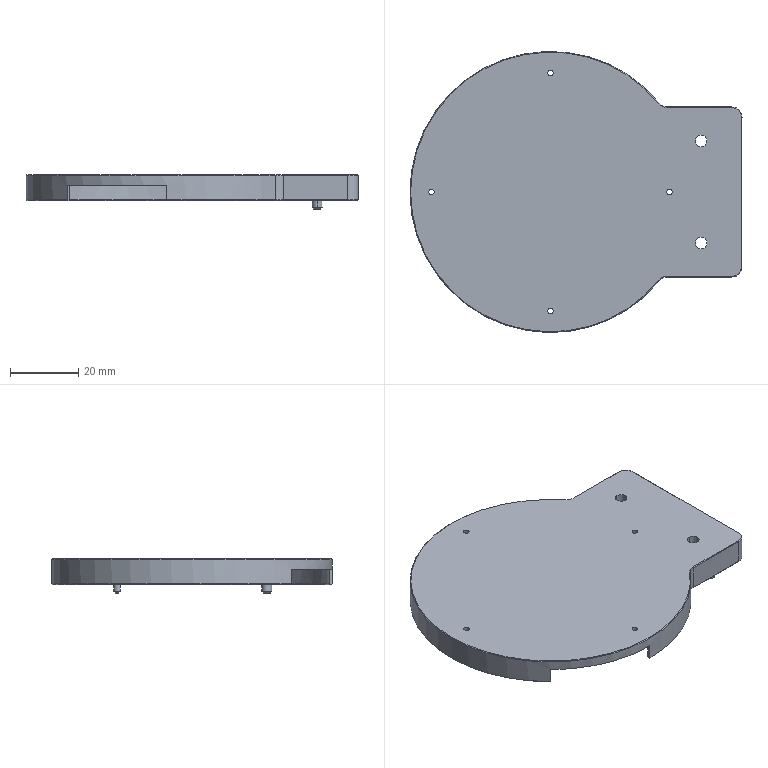NC program | NX | posted with a generic post | part box 97.6 x 82.6 x 10 mm
Whole program:
N10 G17 G21 G94 G90
(DRILLING_COPY_1 , TOOL : D6A45)
N12 T01 M6
N14 G54
N16 G17 G0 G90 X-42.5 Y0. S5000 M3
N18 G43 Z30. H1
N20 G94 G81 G98 Z-1.1 F350. R3.
N22 X-7.5 Y-35.
N24 X36.8 Y-15.
N26 X27.5 Y0.
N28 X36.8 Y15.
N30 X-7.5 Y35.
N32 G80
N34 G0 X-7.5 Y35. Z30.
N36 M5
(DRILLING_COPY_1_COPY_COPY , TOOL : 1.6ZT)
N38 T16 M6
N40 G54
N42 G17 G0 G90 X27.5 Y0. S2000 M3
N44 G43 Z30. H16
N46 G94 G83 G98 Z-4.981 F150. Q2. R3.
N48 X-7.5 Y35.
N50 X-42.5 Y0.
N52 X-7.5 Y-35.
N54 G80
N56 G0 X-7.5 Y-35. Z30.
N58 M5
(DRILLING_COPY_1_COPY_1_1_COPY_1 , TOOL : 3.4ZT)
N60 T03 M6
N62 G54
N64 G17 G0 G90 X36.8 Y15. S2000 M3
N66 G43 Z30. H3
N68 G94 G83 G98 Z-10.021 F200. Q2. R3.
N70 Y-15.
N72 G80
N74 G0 X36.8 Y-15. Z30.
N76 M5
(ZLEVEL_PROFILE , TOOL : D10)
N78 T15 M6
N80 G54
N82 G17 G0 G90 X33.985 Y30.1 S9500 M3
N84 G43 Z30. H15
N86 Z1.5
N88 G94 G1 X45.8 Z0.881 F1000.
N90 X46.498 Z0.844
N92 X48.35 Y29.72 Z0.745
N94 X50.065 Y28.921 Z0.646
N96 X51.549 Y27.749 Z0.547
N98 X52.721 Y26.265 Z0.448
N100 X53.52 Y24.55 Z0.349
N102 X53.9 Y22.698 Z0.25
N104 Y22. Z0.213
N106 Y0. Z-0.94
N108 Y-22. F3200.
N110 G2 X45.8 Y-30.1 R8.1
N112 G1 X27.812
N114 G2 X27.812 Y30.1 R-46.4
N116 G1 X45.8
N118 G2 X53.9 Y22. R8.1
N120 G1 Y0.
N122 Y-21.541 Z-1.316
N124 Y-21.926 Z-1.323
N126 X53.894 Y-22.31 Z-1.329
N128 X53.87 Y-22.694 Z-1.336
N130 X53.828 Y-23.076 Z-1.343
N132 X53.768 Y-23.456 Z-1.35
N134 X53.69 Y-23.833 Z-1.356
N136 X53.594 Y-24.205 Z-1.363
N138 X53.48 Y-24.573 Z-1.37
N140 X53.35 Y-24.935 Z-1.376
N142 X53.202 Y-25.29 Z-1.383
N144 X53.037 Y-25.637 Z-1.39
N146 X52.857 Y-25.977 Z-1.397
N148 X52.66 Y-26.307 Z-1.403
N150 X52.448 Y-26.628 Z-1.41
N152 X52.22 Y-26.939 Z-1.417
N154 X51.979 Y-27.238 Z-1.423
N156 X51.723 Y-27.525 Z-1.43
N158 X51.454 Y-27.8 Z-1.437
N160 X51.172 Y-28.062 Z-1.444
N162 X50.879 Y-28.31 Z-1.45
N164 X50.573 Y-28.544 Z-1.457
N166 X50.257 Y-28.763 Z-1.464
N168 X49.931 Y-28.967 Z-1.47
N170 X49.596 Y-29.156 Z-1.477
N172 X49.252 Y-29.328 Z-1.484
N174 X48.9 Y-29.483 Z-1.491
N176 X48.541 Y-29.622 Z-1.497
N178 X48.176 Y-29.744 Z-1.504
N180 X47.806 Y-29.848 Z-1.511
N182 X47.431 Y-29.934 Z-1.517
N184 X47.053 Y-30.003 Z-1.524
N186 X46.672 Y-30.053 Z-1.531
N188 X46.288 Y-30.085 Z-1.538
N190 X45.904 Y-30.099 Z-1.544
N192 X45.519 Y-30.1 Z-1.551
N194 X28.21 Z-1.853
N196 X27.818 Z-1.86
N198 X27.57 Y-30.382 Z-1.867
N200 X27.317 Y-30.672 Z-1.873
N202 X27.061 Y-30.959 Z-1.88
N204 G2 X27.812 Y30.1 R-46.4
N206 G1 X45.8
N208 G2 X53.9 Y22. R8.1
N210 G1 Y0.
N212 Y-21.541 Z-2.256
N214 Y-21.926 Z-2.263
N216 X53.894 Y-22.31 Z-2.269
N218 X53.87 Y-22.694 Z-2.276
N220 X53.828 Y-23.076 Z-2.283
N222 X53.768 Y-23.456 Z-2.29
N224 X53.69 Y-23.833 Z-2.296
N226 X53.594 Y-24.205 Z-2.303
N228 X53.48 Y-24.573 Z-2.31
N230 X53.35 Y-24.935 Z-2.316
N232 X53.202 Y-25.29 Z-2.323
N234 X53.037 Y-25.637 Z-2.33
N236 X52.857 Y-25.977 Z-2.337
N238 X52.66 Y-26.307 Z-2.343
N240 X52.448 Y-26.628 Z-2.35
N242 X52.22 Y-26.939 Z-2.357
N244 X51.979 Y-27.238 Z-2.363
N246 X51.723 Y-27.525 Z-2.37
N248 X51.454 Y-27.8 Z-2.377
N250 X51.172 Y-28.062 Z-2.384
N252 X50.879 Y-28.31 Z-2.39
N254 X50.573 Y-28.544 Z-2.397
N256 X50.257 Y-28.763 Z-2.404
N258 X49.931 Y-28.967 Z-2.41
N260 X49.596 Y-29.156 Z-2.417
N262 X49.252 Y-29.328 Z-2.424
N264 X48.9 Y-29.483 Z-2.431
N266 X48.541 Y-29.622 Z-2.437
N268 X48.176 Y-29.744 Z-2.444
N270 X47.806 Y-29.848 Z-2.451
N272 X47.431 Y-29.934 Z-2.457
N274 X47.053 Y-30.003 Z-2.464
N276 X46.672 Y-30.053 Z-2.471
N278 X46.288 Y-30.085 Z-2.478
N280 X45.904 Y-30.099 Z-2.484
N282 X45.519 Y-30.1 Z-2.491
N284 X28.21 Z-2.793
N286 X27.818 Z-2.8
N288 X27.57 Y-30.382 Z-2.807
N290 X27.317 Y-30.672 Z-2.813
N292 X27.061 Y-30.959 Z-2.82
N294 G2 X27.812 Y30.1 R-46.4
N296 G1 X45.8
N298 G2 X53.9 Y22. R8.1
N300 G1 Y0.
N302 Y-21.541 Z-3.196
N304 Y-21.926 Z-3.203
N306 X53.894 Y-22.31 Z-3.209
N308 X53.87 Y-22.694 Z-3.216
N310 X53.828 Y-23.076 Z-3.223
N312 X53.768 Y-23.456 Z-3.23
N314 X53.69 Y-23.833 Z-3.236
N316 X53.594 Y-24.205 Z-3.243
N318 X53.48 Y-24.573 Z-3.25
N320 X53.35 Y-24.935 Z-3.256
N322 X53.202 Y-25.29 Z-3.263
N324 X53.037 Y-25.637 Z-3.27
N326 X52.857 Y-25.977 Z-3.277
N328 X52.66 Y-26.307 Z-3.283
N330 X52.448 Y-26.628 Z-3.29
N332 X52.22 Y-26.939 Z-3.297
N334 X51.979 Y-27.238 Z-3.303
N336 X51.723 Y-27.525 Z-3.31
N338 X51.454 Y-27.8 Z-3.317
N340 X51.172 Y-28.062 Z-3.324
N342 X50.879 Y-28.31 Z-3.33
N344 X50.573 Y-28.544 Z-3.337
N346 X50.257 Y-28.763 Z-3.344
N348 X49.931 Y-28.967 Z-3.35
N350 X49.596 Y-29.156 Z-3.357
N352 X49.252 Y-29.328 Z-3.364
N354 X48.9 Y-29.483 Z-3.371
N356 X48.541 Y-29.622 Z-3.377
N358 X48.176 Y-29.744 Z-3.384
N360 X47.806 Y-29.848 Z-3.391
N362 X47.431 Y-29.934 Z-3.397
N364 X47.053 Y-30.003 Z-3.404
N366 X46.672 Y-30.053 Z-3.411
N368 X46.288 Y-30.085 Z-3.418
N370 X45.904 Y-30.099 Z-3.424
N372 X45.519 Y-30.1 Z-3.431
N374 X28.21 Z-3.733
N376 X27.818 Z-3.74
N378 X27.57 Y-30.382 Z-3.747
N380 X27.317 Y-30.672 Z-3.753
N382 X27.061 Y-30.959 Z-3.76
N384 G2 X27.812 Y30.1 R-46.4
N386 G1 X45.8
N388 G2 X53.9 Y22. R8.1
N390 G1 Y0.
N392 Y-21.541 Z-4.136
N394 Y-21.926 Z-4.143
N396 X53.894 Y-22.31 Z-4.149
N398 X53.87 Y-22.694 Z-4.156
N400 X53.828 Y-23.076 Z-4.163
N402 X53.768 Y-23.456 Z-4.17
N404 X53.69 Y-23.833 Z-4.176
N406 X53.594 Y-24.205 Z-4.183
N408 X53.48 Y-24.573 Z-4.19
N410 X53.35 Y-24.935 Z-4.196
N412 X53.202 Y-25.29 Z-4.203
N414 X53.037 Y-25.637 Z-4.21
N416 X52.857 Y-25.977 Z-4.217
N418 X52.66 Y-26.307 Z-4.223
N420 X52.448 Y-26.628 Z-4.23
N422 X52.22 Y-26.939 Z-4.237
N424 X51.979 Y-27.238 Z-4.243
N426 X51.723 Y-27.525 Z-4.25
N428 X51.454 Y-27.8 Z-4.257
N430 X51.172 Y-28.062 Z-4.264
N432 X50.879 Y-28.31 Z-4.27
N434 X50.573 Y-28.544 Z-4.277
N436 X50.257 Y-28.763 Z-4.284
N438 X49.931 Y-28.967 Z-4.29
N440 X49.596 Y-29.156 Z-4.297
N442 X49.252 Y-29.328 Z-4.304
N444 X48.9 Y-29.483 Z-4.311
N446 X48.541 Y-29.622 Z-4.317
N448 X48.176 Y-29.744 Z-4.324
N450 X47.806 Y-29.848 Z-4.331
N452 X47.431 Y-29.934 Z-4.337
N454 X47.053 Y-30.003 Z-4.344
N456 X46.672 Y-30.053 Z-4.351
N458 X46.288 Y-30.085 Z-4.358
N460 X45.904 Y-30.099 Z-4.364
N462 X45.519 Y-30.1 Z-4.371
N464 X28.21 Z-4.673
N466 X27.818 Z-4.68
N468 X27.57 Y-30.382 Z-4.687
N470 X27.317 Y-30.672 Z-4.693
N472 X27.061 Y-30.959 Z-4.7
N474 G2 X27.812 Y30.1 R-46.4
N476 G1 X45.8
N478 G2 X53.9 Y22. R8.1
N480 G1 Y0.
N482 Y-21.541 Z-5.076
N484 Y-21.926 Z-5.083
N486 X53.894 Y-22.31 Z-5.089
N488 X53.87 Y-22.694 Z-5.096
N490 X53.828 Y-23.076 Z-5.103
N492 X53.768 Y-23.456 Z-5.11
N494 X53.69 Y-23.833 Z-5.116
N496 X53.594 Y-24.205 Z-5.123
N498 X53.48 Y-24.573 Z-5.13
N500 X53.35 Y-24.935 Z-5.136
N502 X53.202 Y-25.29 Z-5.143
N504 X53.037 Y-25.637 Z-5.15
N506 X52.857 Y-25.977 Z-5.157
N508 X52.66 Y-26.307 Z-5.163
N510 X52.448 Y-26.628 Z-5.17
N512 X52.22 Y-26.939 Z-5.177
N514 X51.979 Y-27.238 Z-5.183
N516 X51.723 Y-27.525 Z-5.19
N518 X51.454 Y-27.8 Z-5.197
N520 X51.172 Y-28.062 Z-5.204
N522 X50.879 Y-28.31 Z-5.21
N524 X50.573 Y-28.544 Z-5.217
N526 X50.257 Y-28.763 Z-5.224
N528 X49.931 Y-28.967 Z-5.23
N530 X49.596 Y-29.156 Z-5.237
N532 X49.252 Y-29.328 Z-5.244
N534 X48.9 Y-29.483 Z-5.251
N536 X48.541 Y-29.622 Z-5.257
N538 X48.176 Y-29.744 Z-5.264
N540 X47.806 Y-29.848 Z-5.271
N542 X47.431 Y-29.934 Z-5.277
N544 X47.053 Y-30.003 Z-5.284
N546 X46.672 Y-30.053 Z-5.291
N548 X46.288 Y-30.085 Z-5.298
N550 X45.904 Y-30.099 Z-5.304
N552 X45.519 Y-30.1 Z-5.311
N554 X28.21 Z-5.613
N556 X27.818 Z-5.62
N558 X27.57 Y-30.382 Z-5.627
N560 X27.317 Y-30.672 Z-5.633
N562 X27.061 Y-30.959 Z-5.64
N564 G2 X27.812 Y30.1 R-46.4
N566 G1 X45.8
N568 G2 X53.9 Y22. R8.1
N570 G1 Y0.
N572 Y-21.541 Z-6.016
N574 Y-21.926 Z-6.023
N576 X53.894 Y-22.31 Z-6.029
N578 X53.87 Y-22.694 Z-6.036
N580 X53.828 Y-23.076 Z-6.043
N582 X53.768 Y-23.456 Z-6.05
N584 X53.69 Y-23.833 Z-6.056
N586 X53.594 Y-24.205 Z-6.063
N588 X53.48 Y-24.573 Z-6.07
N590 X53.35 Y-24.935 Z-6.076
N592 X53.202 Y-25.29 Z-6.083
N594 X53.037 Y-25.637 Z-6.09
N596 X52.857 Y-25.977 Z-6.097
N598 X52.66 Y-26.307 Z-6.103
N600 X52.448 Y-26.628 Z-6.11
N602 X52.22 Y-26.939 Z-6.117
N604 X51.979 Y-27.238 Z-6.123
N606 X51.723 Y-27.525 Z-6.13
N608 X51.454 Y-27.8 Z-6.137
N610 X51.172 Y-28.062 Z-6.144
N612 X50.879 Y-28.31 Z-6.15
N614 X50.573 Y-28.544 Z-6.157
N616 X50.257 Y-28.763 Z-6.164
N618 X49.931 Y-28.967 Z-6.17
N620 X49.596 Y-29.156 Z-6.177
N622 X49.252 Y-29.328 Z-6.184
N624 X48.9 Y-29.483 Z-6.191
N626 X48.541 Y-29.622 Z-6.197
N628 X48.176 Y-29.744 Z-6.204
N630 X47.806 Y-29.848 Z-6.211
N632 X47.431 Y-29.934 Z-6.217
N634 X47.053 Y-30.003 Z-6.224
N636 X46.672 Y-30.053 Z-6.231
N638 X46.288 Y-30.085 Z-6.238
N640 X45.904 Y-30.099 Z-6.244
N642 X45.519 Y-30.1 Z-6.251
N644 X28.21 Z-6.553
N646 X27.818 Z-6.56
N648 X27.57 Y-30.382 Z-6.567
N650 X27.317 Y-30.672 Z-6.573
N652 X27.061 Y-30.959 Z-6.58
N654 G2 X27.812 Y30.1 R-46.4
N656 G1 X45.8
N658 G2 X53.9 Y22. R8.1
N660 G1 Y0.
N662 Y-21.541 Z-6.956
N664 Y-21.926 Z-6.963
N666 X53.894 Y-22.31 Z-6.969
N668 X53.87 Y-22.694 Z-6.976
N670 X53.828 Y-23.076 Z-6.983
N672 X53.768 Y-23.456 Z-6.99
N674 X53.69 Y-23.833 Z-6.996
N676 X53.594 Y-24.205 Z-7.003
N678 X53.48 Y-24.573 Z-7.01
N680 X53.35 Y-24.935 Z-7.016
N682 X53.202 Y-25.29 Z-7.023
N684 X53.037 Y-25.637 Z-7.03
N686 X52.857 Y-25.977 Z-7.037
N688 X52.66 Y-26.307 Z-7.043
N690 X52.448 Y-26.628 Z-7.05
N692 X52.22 Y-26.939 Z-7.057
N694 X51.979 Y-27.238 Z-7.063
N696 X51.723 Y-27.525 Z-7.07
N698 X51.454 Y-27.8 Z-7.077
N700 X51.172 Y-28.062 Z-7.084
N702 X50.879 Y-28.31 Z-7.09
N704 X50.573 Y-28.544 Z-7.097
N706 X50.257 Y-28.763 Z-7.104
N708 X49.931 Y-28.967 Z-7.11
N710 X49.596 Y-29.156 Z-7.117
N712 X49.252 Y-29.328 Z-7.124
N714 X48.9 Y-29.483 Z-7.131
N716 X48.541 Y-29.622 Z-7.137
N718 X48.176 Y-29.744 Z-7.144
N720 X47.806 Y-29.848 Z-7.151
N722 X47.431 Y-29.934 Z-7.157
N724 X47.053 Y-30.003 Z-7.164
N726 X46.672 Y-30.053 Z-7.171
N728 X46.288 Y-30.085 Z-7.178
N730 X45.904 Y-30.099 Z-7.184
N732 X45.519 Y-30.1 Z-7.191
N734 X28.21 Z-7.493
N736 X27.818 Z-7.5
N738 X27.57 Y-30.382 Z-7.507
N740 X27.317 Y-30.672 Z-7.513
N742 X27.061 Y-30.959 Z-7.52
N744 G2 X27.812 Y30.1 R-46.4
N746 G1 X45.8
N748 G2 X53.9 Y22. R8.1
N750 G1 Y0.
N752 Y-21.541 Z-7.896
N754 Y-21.926 Z-7.903
N756 X53.894 Y-22.31 Z-7.909
N758 X53.87 Y-22.694 Z-7.916
N760 X53.828 Y-23.076 Z-7.923
N762 X53.768 Y-23.456 Z-7.93
N764 X53.69 Y-23.833 Z-7.936
N766 X53.594 Y-24.205 Z-7.943
N768 X53.48 Y-24.573 Z-7.95
N770 X53.35 Y-24.935 Z-7.956
N772 X53.202 Y-25.29 Z-7.963
N774 X53.037 Y-25.637 Z-7.97
N776 X52.857 Y-25.977 Z-7.977
N778 X52.66 Y-26.307 Z-7.983
N780 X52.448 Y-26.628 Z-7.99
N782 X52.22 Y-26.939 Z-7.997
N784 X51.979 Y-27.238 Z-8.003
N786 X51.723 Y-27.525 Z-8.01
N788 X51.454 Y-27.8 Z-8.017
N790 X51.172 Y-28.062 Z-8.024
N792 X50.879 Y-28.31 Z-8.03
N794 X50.573 Y-28.544 Z-8.037
N796 X50.257 Y-28.763 Z-8.044
N798 X49.931 Y-28.967 Z-8.05
N800 X49.596 Y-29.156 Z-8.057
N802 X49.252 Y-29.328 Z-8.064
N804 X48.9 Y-29.483 Z-8.071
N806 X48.541 Y-29.622 Z-8.077
N808 X48.176 Y-29.744 Z-8.084
N810 X47.806 Y-29.848 Z-8.091
N812 X47.431 Y-29.934 Z-8.097
N814 X47.053 Y-30.003 Z-8.104
N816 X46.672 Y-30.053 Z-8.111
N818 X46.288 Y-30.085 Z-8.118
N820 X45.904 Y-30.099 Z-8.124
N822 X45.519 Y-30.1 Z-8.131
N824 X28.21 Z-8.433
N826 X27.818 Z-8.44
N828 X27.57 Y-30.382 Z-8.447
N830 X27.317 Y-30.672 Z-8.453
N832 X27.061 Y-30.959 Z-8.46
N834 G2 X27.812 Y30.1 R-46.4
N836 G1 X45.8
N838 G2 X53.9 Y22. R8.1
N840 G1 Y0.
N842 Y-21.541 Z-8.836
N844 Y-21.926 Z-8.843
N846 X53.894 Y-22.31 Z-8.849
N848 X53.87 Y-22.694 Z-8.856
N850 X53.828 Y-23.076 Z-8.863
N852 X53.768 Y-23.456 Z-8.87
N854 X53.69 Y-23.833 Z-8.876
N856 X53.594 Y-24.205 Z-8.883
N858 X53.48 Y-24.573 Z-8.89
N860 X53.35 Y-24.935 Z-8.896
N862 X53.202 Y-25.29 Z-8.903
N864 X53.037 Y-25.637 Z-8.91
N866 X52.857 Y-25.977 Z-8.917
N868 X52.66 Y-26.307 Z-8.923
N870 X52.448 Y-26.628 Z-8.93
N872 X52.22 Y-26.939 Z-8.937
N874 X51.979 Y-27.238 Z-8.943
N876 X51.723 Y-27.525 Z-8.95
N878 X51.454 Y-27.8 Z-8.957
N880 X51.172 Y-28.062 Z-8.964
N882 X50.879 Y-28.31 Z-8.97
N884 X50.573 Y-28.544 Z-8.977
N886 X50.257 Y-28.763 Z-8.984
N888 X49.931 Y-28.967 Z-8.99
N890 X49.596 Y-29.156 Z-8.997
N892 X49.252 Y-29.328 Z-9.004
N894 X48.9 Y-29.483 Z-9.011
N896 X48.541 Y-29.622 Z-9.017
N898 X48.176 Y-29.744 Z-9.024
N900 X47.806 Y-29.848 Z-9.031
N902 X47.431 Y-29.934 Z-9.037
N904 X47.053 Y-30.003 Z-9.044
N906 X46.672 Y-30.053 Z-9.051
N908 X46.288 Y-30.085 Z-9.058
N910 X45.904 Y-30.099 Z-9.064
N912 X45.519 Y-30.1 Z-9.071
N914 X28.21 Z-9.373
N916 X27.818 Z-9.38
N918 X27.57 Y-30.382 Z-9.387
N920 X27.317 Y-30.672 Z-9.393
N922 X27.061 Y-30.959 Z-9.4
N924 G2 X27.812 Y30.1 R-46.4
N926 G1 X45.8
N928 G2 X53.9 Y22. R8.1
N930 G1 Y-22.
N932 G2 X45.8 Y-30.1 R8.1
N934 G1 X27.812
N936 G2 X27.061 Y-30.959 R46.4
N938 G1 Z-7.9
N940 G0 Z30.
N942 M5
(ZLEVEL_PROFILE_2 , TOOL : D6)
N944 T12 M6
N946 G54
N948 G17 G0 G90 X26.467 Y30.274 S9500 M3
N950 G43 Z30. H12
N952 Z-0.5
N954 G94 G1 X26.123 Y29.307 F1600.
N956 G3 X26.231 Y28.717 R0.6
N958 G2 X26.829 Y28. R44.3
N960 G1 X27.772
N962 G3 X28.292 Y28.3 R0.6
N964 G1 X28.812 Y29.2
N966 G0 X26.467 Y30.274 Z-1.
N968 G1 X26.123 Y29.307
N970 G3 X26.231 Y28.717 R0.6
N972 G2 X26.829 Y28. R44.3
N974 G1 X27.772
N976 G3 X28.292 Y28.3 R0.6
N978 G1 X28.812 Y29.2
N980 G0 X26.467 Y30.274 Z-1.5
N982 G1 X26.123 Y29.307
N984 G3 X26.231 Y28.717 R0.6
N986 G2 X26.829 Y28. R44.3
N988 G1 X27.772
N990 G3 X28.292 Y28.3 R0.6
N992 G1 X28.812 Y29.2
N994 G0 X26.467 Y30.274 Z-2.
N996 G1 X26.123 Y29.307
N998 G3 X26.231 Y28.717 R0.6
N1000 G2 X26.829 Y28. R44.3
N1002 G1 X27.772
N1004 G3 X28.292 Y28.3 R0.6
N1006 G1 X28.812 Y29.2
N1008 G0 X26.467 Y30.274 Z-2.5
N1010 G1 X26.123 Y29.307
N1012 G3 X26.231 Y28.717 R0.6
N1014 G2 X26.829 Y28. R44.3
N1016 G1 X27.772
N1018 G3 X28.292 Y28.3 R0.6
N1020 G1 X28.812 Y29.2
N1022 G0 X26.467 Y30.274 Z-3.
N1024 G1 X26.123 Y29.307
N1026 G3 X26.231 Y28.717 R0.6
N1028 G2 X26.829 Y28. R44.3
N1030 G1 X27.772
N1032 G3 X28.292 Y28.3 R0.6
N1034 G1 X28.812 Y29.2
N1036 G0 X26.467 Y30.274 Z-3.5
N1038 G1 X26.123 Y29.307
N1040 G3 X26.231 Y28.717 R0.6
N1042 G2 X26.829 Y28. R44.3
N1044 G1 X27.772
N1046 G3 X28.292 Y28.3 R0.6
N1048 G1 X28.812 Y29.2
N1050 G0 X26.467 Y30.274 Z-4.
N1052 G1 X26.123 Y29.307
N1054 G3 X26.231 Y28.717 R0.6
N1056 G2 X26.829 Y28. R44.3
N1058 G1 X27.772
N1060 G3 X28.292 Y28.3 R0.6
N1062 G1 X28.812 Y29.2
N1064 G0 X26.467 Y30.274 Z-4.5
N1066 G1 X26.123 Y29.307
N1068 G3 X26.231 Y28.717 R0.6
N1070 G2 X26.829 Y28. R44.3
N1072 G1 X27.772
N1074 G3 X28.292 Y28.3 R0.6
N1076 G1 X28.812 Y29.2
N1078 G0 X26.467 Y30.274 Z-5.
N1080 G1 X26.123 Y29.307
N1082 G3 X26.231 Y28.717 R0.6
N1084 G2 X26.829 Y28. R44.3
N1086 G1 X27.772
N1088 G3 X28.292 Y28.3 R0.6
N1090 G1 X28.812 Y29.2
N1092 G0 X26.467 Y30.274 Z-5.5
N1094 G1 X26.123 Y29.307
N1096 G3 X26.231 Y28.717 R0.6
N1098 G2 X26.829 Y28. R44.3
N1100 G1 X27.772
N1102 G3 X28.292 Y28.3 R0.6
N1104 G1 X28.812 Y29.2
N1106 G0 X26.467 Y30.274 Z-6.
N1108 G1 X26.123 Y29.307
N1110 G3 X26.231 Y28.717 R0.6
N1112 G2 X26.829 Y28. R44.3
N1114 G1 X27.772
N1116 G3 X28.292 Y28.3 R0.6
N1118 G1 X28.812 Y29.2
N1120 G0 X26.467 Y30.274 Z-6.5
N1122 G1 X26.123 Y29.307
N1124 G3 X26.231 Y28.717 R0.6
N1126 G2 X26.829 Y28. R44.3
N1128 G1 X27.772
N1130 G3 X28.292 Y28.3 R0.6
N1132 G1 X28.812 Y29.2
N1134 G0 X26.467 Y30.274 Z-7.
N1136 G1 X26.123 Y29.307
N1138 G3 X26.231 Y28.717 R0.6
N1140 G2 X26.829 Y28. R44.3
N1142 G1 X27.772
N1144 G3 X28.292 Y28.3 R0.6
N1146 G1 X28.812 Y29.2
N1148 G0 Z30.
N1150 Y-29.2
N1152 Z-0.5
N1154 G1 X28.292 Y-28.3
N1156 G3 X27.772 Y-28. R0.6
N1158 G1 X26.829
N1160 G2 X26.231 Y-28.717 R44.3
N1162 G3 X26.123 Y-29.307 R0.6
N1164 G1 X26.467 Y-30.274
N1166 G0 X28.812 Y-29.2 Z-1.
N1168 G1 X28.292 Y-28.3
N1170 G3 X27.772 Y-28. R0.6
N1172 G1 X26.829
N1174 G2 X26.231 Y-28.717 R44.3
N1176 G3 X26.123 Y-29.307 R0.6
N1178 G1 X26.467 Y-30.274
N1180 G0 X28.812 Y-29.2 Z-1.5
N1182 G1 X28.292 Y-28.3
N1184 G3 X27.772 Y-28. R0.6
N1186 G1 X26.829
N1188 G2 X26.231 Y-28.717 R44.3
N1190 G3 X26.123 Y-29.307 R0.6
N1192 G1 X26.467 Y-30.274
N1194 G0 X28.812 Y-29.2 Z-2.
N1196 G1 X28.292 Y-28.3
N1198 G3 X27.772 Y-28. R0.6
N1200 G1 X26.829
N1202 G2 X26.231 Y-28.717 R44.3
N1204 G3 X26.123 Y-29.307 R0.6
N1206 G1 X26.467 Y-30.274
N1208 G0 X28.812 Y-29.2 Z-2.5
N1210 G1 X28.292 Y-28.3
N1212 G3 X27.772 Y-28. R0.6
N1214 G1 X26.829
N1216 G2 X26.231 Y-28.717 R44.3
N1218 G3 X26.123 Y-29.307 R0.6
N1220 G1 X26.467 Y-30.274
N1222 G0 X28.812 Y-29.2 Z-3.
N1224 G1 X28.292 Y-28.3
N1226 G3 X27.772 Y-28. R0.6
N1228 G1 X26.829
N1230 G2 X26.231 Y-28.717 R44.3
N1232 G3 X26.123 Y-29.307 R0.6
N1234 G1 X26.467 Y-30.274
N1236 G0 X28.812 Y-29.2 Z-3.5
N1238 G1 X28.292 Y-28.3
N1240 G3 X27.772 Y-28. R0.6
N1242 G1 X26.829
N1244 G2 X26.231 Y-28.717 R44.3
N1246 G3 X26.123 Y-29.307 R0.6
N1248 G1 X26.467 Y-30.274
N1250 G0 X28.812 Y-29.2 Z-4.
N1252 G1 X28.292 Y-28.3
N1254 G3 X27.772 Y-28. R0.6
N1256 G1 X26.829
N1258 G2 X26.231 Y-28.717 R44.3
N1260 G3 X26.123 Y-29.307 R0.6
N1262 G1 X26.467 Y-30.274
N1264 G0 X28.812 Y-29.2 Z-4.5
N1266 G1 X28.292 Y-28.3
N1268 G3 X27.772 Y-28. R0.6
N1270 G1 X26.829
N1272 G2 X26.231 Y-28.717 R44.3
N1274 G3 X26.123 Y-29.307 R0.6
N1276 G1 X26.467 Y-30.274
N1278 G0 X28.812 Y-29.2 Z-5.
N1280 G1 X28.292 Y-28.3
N1282 G3 X27.772 Y-28. R0.6
N1284 G1 X26.829
N1286 G2 X26.231 Y-28.717 R44.3
N1288 G3 X26.123 Y-29.307 R0.6
N1290 G1 X26.467 Y-30.274
N1292 G0 X28.812 Y-29.2 Z-5.5
N1294 G1 X28.292 Y-28.3
N1296 G3 X27.772 Y-28. R0.6
N1298 G1 X26.829
N1300 G2 X26.231 Y-28.717 R44.3
N1302 G3 X26.123 Y-29.307 R0.6
N1304 G1 X26.467 Y-30.274
N1306 G0 X28.812 Y-29.2 Z-6.
N1308 G1 X28.292 Y-28.3
N1310 G3 X27.772 Y-28. R0.6
N1312 G1 X26.829
N1314 G2 X26.231 Y-28.717 R44.3
N1316 G3 X26.123 Y-29.307 R0.6
N1318 G1 X26.467 Y-30.274
N1320 G0 X28.812 Y-29.2 Z-6.5
N1322 G1 X28.292 Y-28.3
N1324 G3 X27.772 Y-28. R0.6
N1326 G1 X26.829
N1328 G2 X26.231 Y-28.717 R44.3
N1330 G3 X26.123 Y-29.307 R0.6
N1332 G1 X26.467 Y-30.274
N1334 G0 X28.812 Y-29.2 Z-7.
N1336 G1 X28.292 Y-28.3
N1338 G3 X27.772 Y-28. R0.6
N1340 G1 X26.829
N1342 G2 X26.231 Y-28.717 R44.3
N1344 G3 X26.123 Y-29.307 R0.6
N1346 G1 X26.467 Y-30.274
N1348 G0 Z30.
N1350 M5
(PLANAR_MILL_COPY_COPY_COPY_COPY_COPY_COPY_1_COPY_1 , TOOL : D6A45)
N1352 T01 M6
N1354 G54
N1356 G17 G0 G90 X50.1 Y0.866 S9500 M3
N1358 G43 Z30. H1
N1360 Z0.5
N1362 G94 G1 Z-1. F1250.
N1364 G3 X49.6 Y0. R1.
N1366 G1 Y-22.
N1368 G2 X45.8 Y-25.8 R3.8
N1370 G1 X26.829
N1372 G3 X25.124 Y-26.609 R2.2
N1374 G2 X25.124 Y26.609 R-42.1
N1376 G3 X26.829 Y25.8 R2.2
N1378 G1 X45.8
N1380 G2 X49.6 Y22. R3.8
N1382 G1 Y0.
N1384 G3 X50.1 Y-0.866 R1.
N1386 G1 Z0.5
N1388 G0 Z30.
N1390 X37.45 Y14.567
N1392 Z0.5
N1394 G1 Z-1.
N1396 G3 X37.7 Y15. R0.5
N1398 X36.8 Y15.9 R0.9
N1400 X37.7 Y15. R-0.9
N1402 X37.45 Y15.433 R0.5
N1404 G1 Z0.5
N1406 G0 Z30.
N1408 Y-15.433
N1410 Z0.5
N1412 G1 Z-1.
N1414 G3 X37.7 Y-15. R0.5
N1416 X36.8 Y-14.1 R0.9
N1418 X37.7 Y-15. R-0.9
N1420 X37.45 Y-14.567 R0.5
N1422 G1 Z0.5
N1424 G0 Z30.
N1426 M5
(ZLEVEL_PROFILE_COPY_1_COPY_COPY_1_COPY_COPY , TOOL : D10JING)
N1428 T14 M6
N1430 G54
N1432 G17 G0 G90 X53.98 Y22.572 S9500 M3
N1434 G43 Z30. H14
N1436 Z-8.525
N1438 G94 G1 Z-9.525 F1000.
N1440 G3 X53.8 Y22. R1.
N1442 G1 Y-22. F1200.
N1444 G2 X45.8 Y-30. R8.
N1446 G1 X27.766
N1448 G2 X27.766 Y30. R-46.3
N1450 G1 X45.8
N1452 G2 X53.8 Y22. R8.
N1454 G1 Y14.839 Z-9.65
N1456 Y-22.
N1458 G2 X45.8 Y-30. R8.
N1460 G1 X27.766
N1462 G2 X27.766 Y30. R-46.3
N1464 G1 X45.8
N1466 G2 X53.8 Y22. R8.
N1468 G1 Y14.839 Z-9.775
N1470 Y-22.
N1472 G2 X45.8 Y-30. R8.
N1474 G1 X27.766
N1476 G2 X27.766 Y30. R-46.3
N1478 G1 X45.8
N1480 G2 X53.8 Y22. R8.
N1482 G1 Y14.839 Z-9.9
N1484 Y-22.
N1486 G2 X45.8 Y-30. R8.
N1488 G1 X27.766
N1490 G2 X27.766 Y30. R-46.3
N1492 G1 X45.8
N1494 G2 X53.8 Y22. R8.
N1496 G1 Y14.839
N1498 G3 X54. Y14.239 R1.
N1500 G1 Z-8.9
N1502 G0 Z30.
N1504 M5
N1506 M2